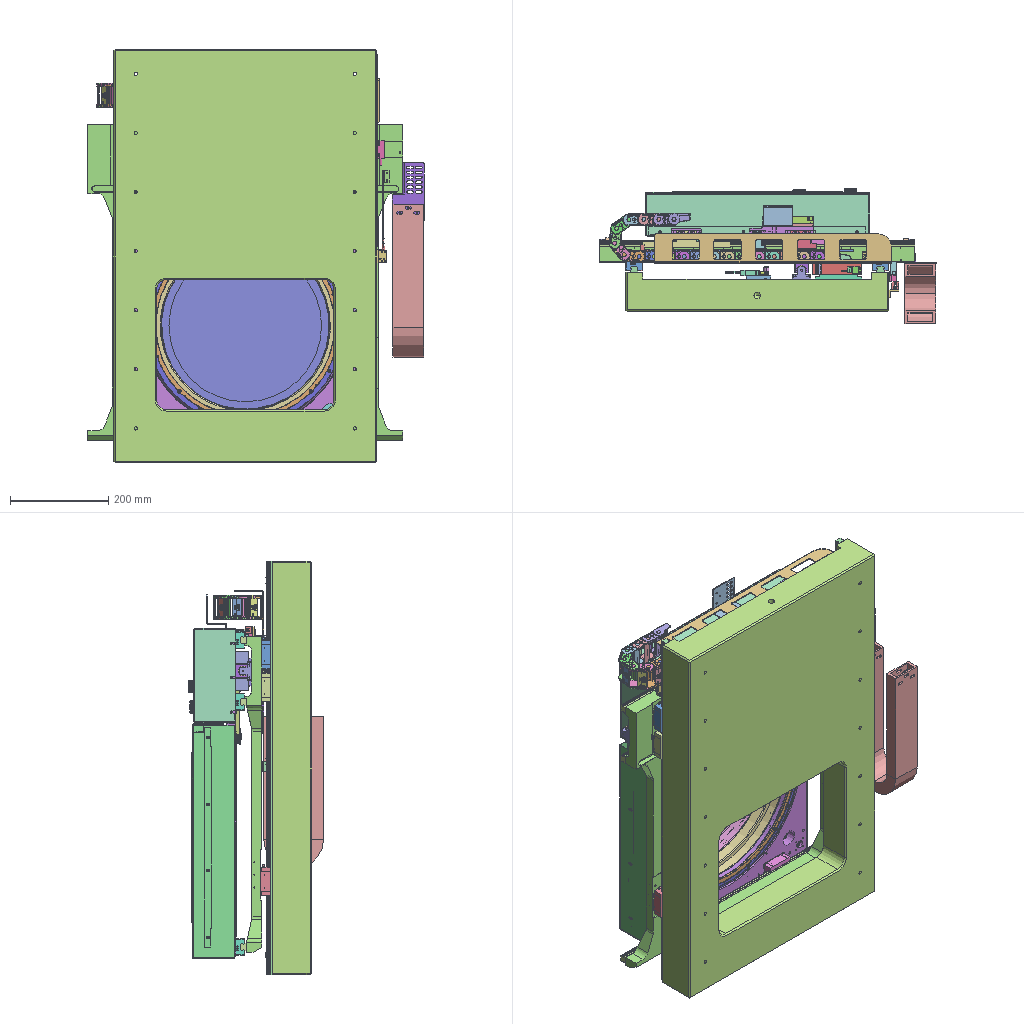Assembly | NX | 123 different items | 296 placed | box 684 x 274 x 840 mm
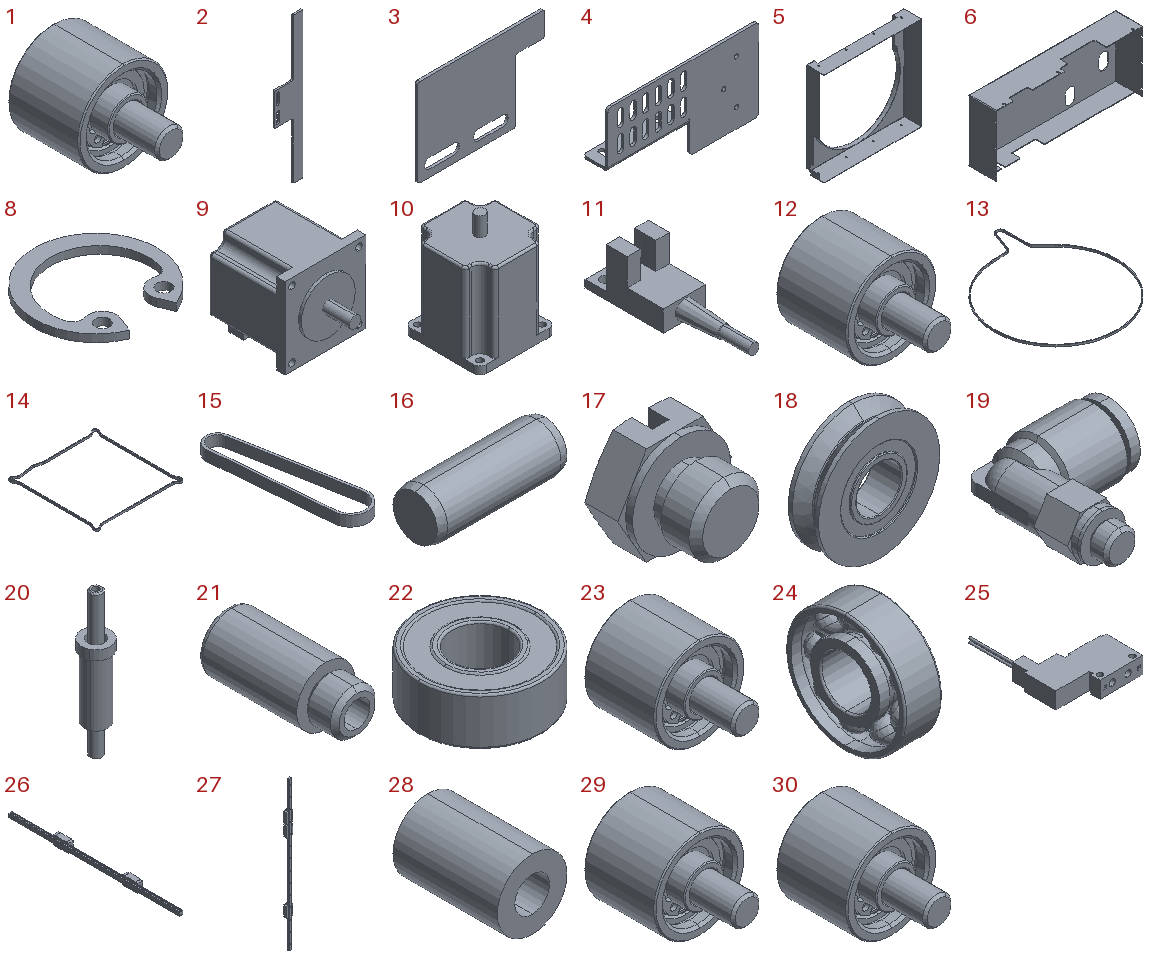Parts list (item | quantity | parent item | size | volume | features):
1 | x1 | in 56 | 19 x 27 x 19 mm | 4161 mm3 | features BREP 6
2 | x1 | in 56 | 35 x 2 x 180 mm | 5942 mm3 | features BREP 1
3 | x1 | in 56 | 52 x 1 x 36 mm | 1447 mm3 | features BREP 1
4 | x1 | in 50 | 120 x 20 x 65 mm | 13263 mm3 | features BREP 1
5 | x1 | in 34 | 477 x 86 x 455 mm | 309171 mm3 | features BREP 1
6 | x1 | in 34 | 456 x 85 x 191 mm | 341001 mm3 | features BREP 1
7 | x1 | in 48 | - | - | features BREP 42
8 | x11 | in 1, 12, 23, 29, 30, 31, 32, 33, 57, 59, 113 | 13 x 12.505 x 0.8 mm | 39.691 mm3 | features BREP 1
9 | x1 | in 62 | 57 x 90 x 65 mm | 164072 mm3 | features BREP 1
10 | x1 | in 35 | 60 x 60 x 105.1 mm | 217707 mm3 | features BREP 1
11 | x3 | in 49, 50 | 14 x 49 x 16 mm | 2990 mm3 | features BREP 1
12 | x1 | in 56 | 19 x 27 x 19 mm | 4161 mm3 | features BREP 6
13 | x1 | in 61 | 398.69 x 477.38 x 6 mm | 16623 mm3 | features BREP 1
14 | x1 | in 56 | 431.47 x 436.47 x 9 mm | 59188 mm3 | features BREP 1
15 | x1 | in 56 | 38.615 x 126.615 x 9 mm | 4997 mm3 | features BREP 1
16 | x6 | in 61 | 8 x 3 x 3 mm | 55.936 mm3 | features BREP 1
17 | x1 | in 64 | 8.083 x 6.5 x 7 mm | 172.44 mm3 | features BREP 1
18 | x10 | in 37, 38, 39, 40, 41, 42, 43, 44, 45, 46 | 16 x 4 x 16 mm | 572.042 mm3 | features BREP 1
19 | x1 | in 64 | 18.541 x 21.7 x 10.4 mm | 1291 mm3 | features BREP 1
20 | x4 | in 61 | 12 x 12 x 60 mm | 2642 mm3 | features BREP 2
21 | x1 | in 64 | 6.5 x 15 x 6.5 mm | 404.687 mm3 | features BREP 1
22 | x22 | in 1, 12, 23, 29, 30, 31, 32, 33, 57, 59, 60, 113 | 13 x 13 x 5 mm | 502.459 mm3 | features BREP 1
23 | x1 | in 56 | 19 x 27 x 19 mm | 4161 mm3 | features BREP 6
24 | x8 | in 52, 53, 54, 55 | 6 x 19 x 19 mm | 760.399 mm3 | features BREP 3
25 | x1 | in 64 | 49.5 x 69.5 x 11 mm | 13145 mm3 | features BREP 1
26 | x3 | in 50 | 24 x 640 x 34 mm | 168254 mm3 | features BREP 3
27 | x2 | in 49 | 34 x 24 x 840 mm | 231169 mm3 | features BREP 4
28 | x4 | in 102 | 8 x 12 x 8 mm | 452.389 mm3 | features BREP 1
29 | x1 | in 56 | 19 x 27 x 19 mm | 4161 mm3 | features BREP 6
30 | x1 | in 56 | 19 x 27 x 19 mm | 4161 mm3 | features BREP 6
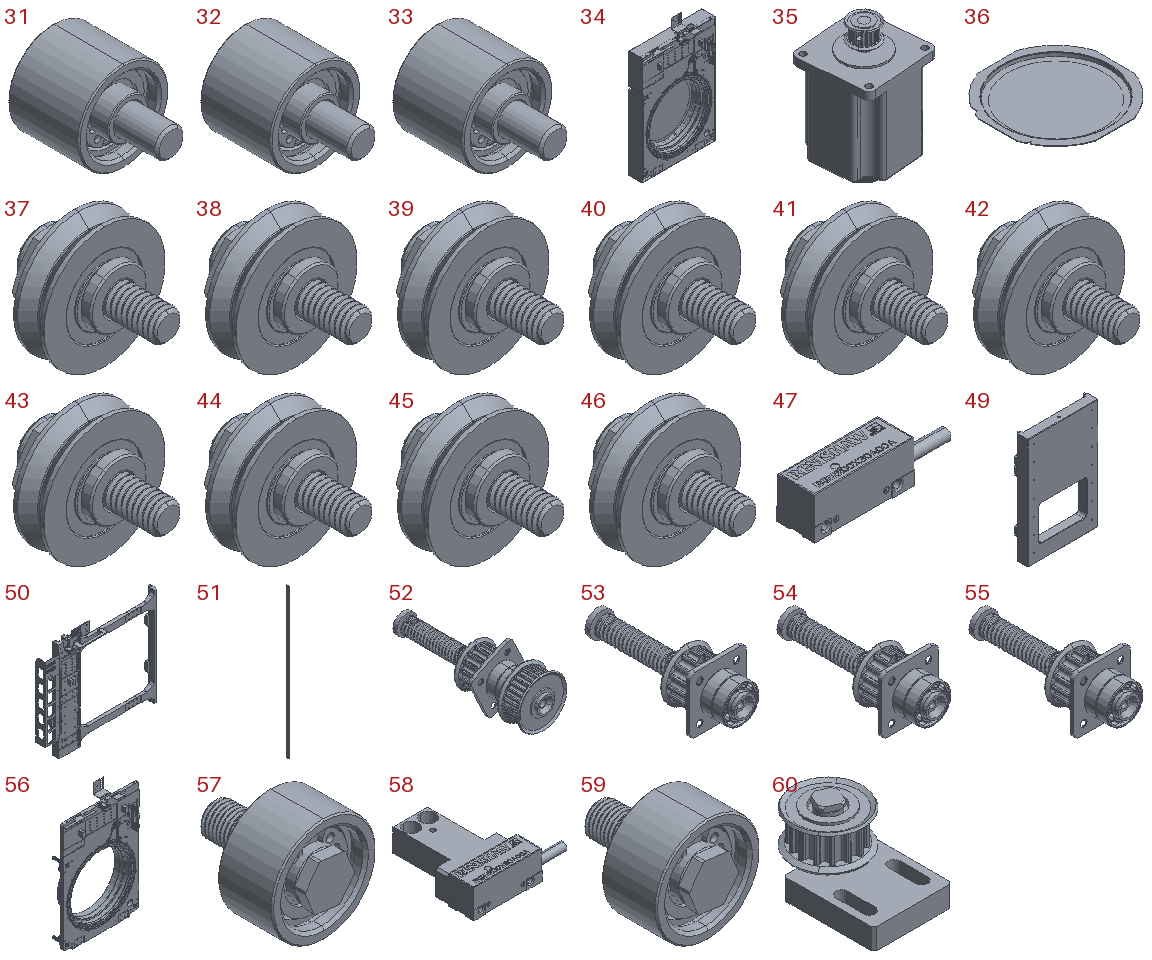31 | x1 | in 56 | 19 x 27 x 19 mm | 4161 mm3 | features BREP 6
32 | x1 | in 56 | 19 x 27 x 19 mm | 4161 mm3 | features BREP 6
33 | x1 | in 56 | 19 x 27 x 19 mm | 4161 mm3 | features BREP 6
34 | x1 | - | - | 6738834 mm3 | features BREP 68
35 | x1 | in 56 | 64.01 x 64.01 x 105.5 mm | 224733 mm3 | features BREP 3
36 | x1 | in 102 | 380 x 380 x 12.65 mm | 79362 mm3 | features BREP 2
37 | x1 | in 56 | 16 x 17 x 16 mm | 1088 mm3 | features BREP 4
38 | x1 | in 56 | 16 x 17 x 16 mm | 1088 mm3 | features BREP 4
39 | x1 | in 56 | 16 x 17 x 16 mm | 1088 mm3 | features BREP 4
40 | x1 | in 56 | 16 x 17 x 16 mm | 1088 mm3 | features BREP 4
41 | x1 | in 102 | 16 x 17 x 16 mm | 1088 mm3 | features BREP 4
42 | x1 | in 102 | 16 x 17 x 16 mm | 1088 mm3 | features BREP 4
43 | x1 | in 102 | 16 x 17 x 16 mm | 1088 mm3 | features BREP 4
44 | x1 | in 102 | 16 x 17 x 16 mm | 1088 mm3 | features BREP 4
45 | x1 | in 102 | 16 x 17 x 16 mm | 1088 mm3 | features BREP 4
46 | x1 | in 56 | 16 x 17 x 16 mm | 1088 mm3 | features BREP 4
47 | x2 | in 58, 69 | 50.65 x 13.5 x 14.8 mm | 6947 mm3 | features BREP 1
48 | x1 | - | - | - | features BREP 92
49 | x1 | in 48 | 555 x 105 x 840 mm | 24900873 mm3 | features BREP 22
50 | x1 | in 48 | - | 4255848 mm3 | features BREP 27
51 | x2 | in 49, 50 | 0.3 x 6 x 390 mm | 702 mm3 | features BREP 1
52 | x1 | in 56 | 37.314 x 92.5 x 37.314 mm | 18812 mm3 | features BREP 11
53 | x1 | in 56 | 29.5 x 77 x 29.5 mm | 11213 mm3 | features BREP 9
54 | x1 | in 56 | 29.5 x 77 x 29.5 mm | 11213 mm3 | features BREP 9
55 | x1 | in 56 | 29.5 x 77 x 29.5 mm | 11213 mm3 | features BREP 9
56 | x1 | in 34 | - | 4419914 mm3 | features BREP 53
57 | x1 | in 61 | 19 x 21 x 19 mm | 2699 mm3 | features BREP 6
58 | x1 | in 56 | 50.65 x 50.5 x 14.8 mm | 15333 mm3 | features BREP 2
59 | x1 | in 61 | 19 x 21 x 19 mm | 2699 mm3 | features BREP 6
60 | x1 | in 56 | 30 x 46 x 27.5 mm | 12594 mm3 | features BREP 6
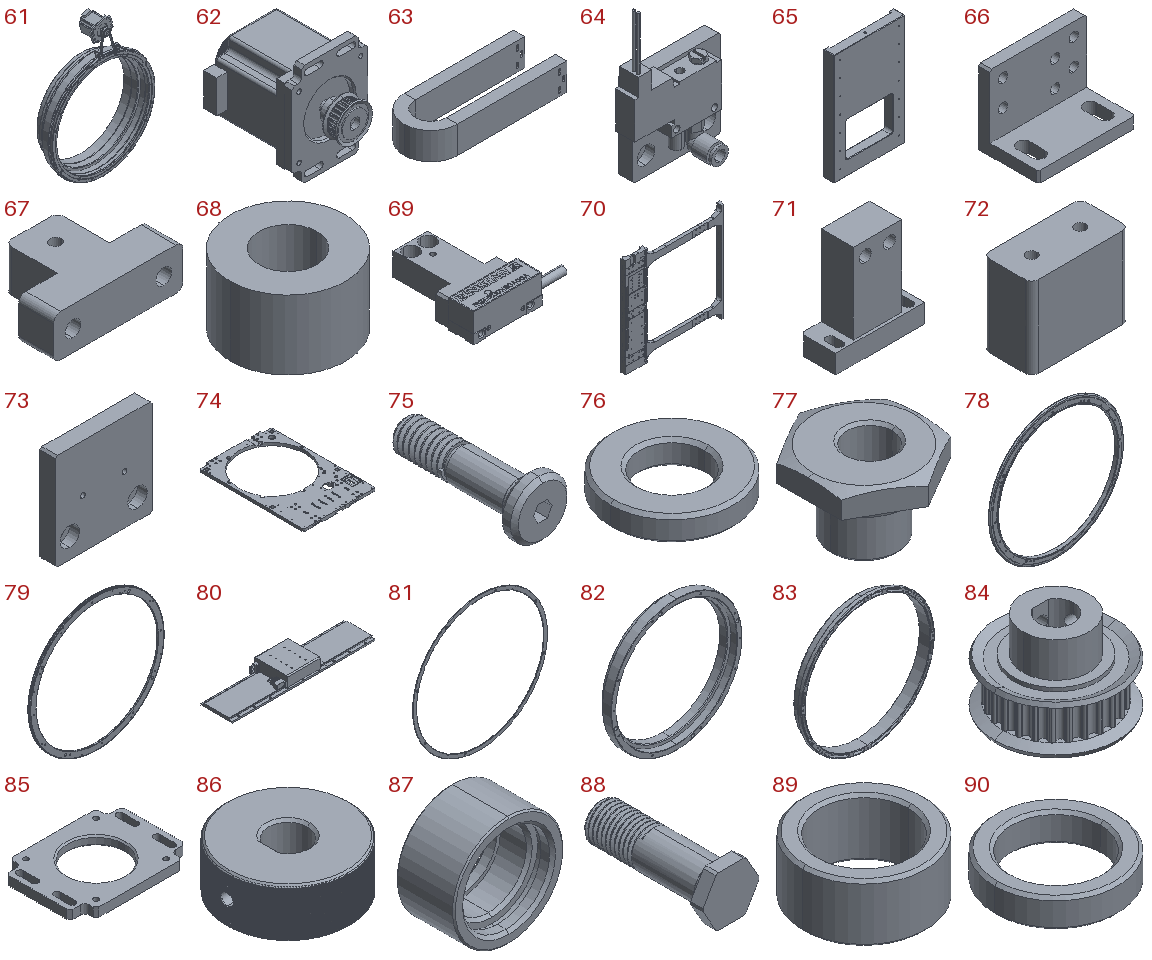61 | x1 | in 56 | - | 1411287 mm3 | features BREP 19
62 | x1 | in 61 | 65.5 x 93.95 x 78 mm | 190120 mm3 | features BREP 4
63 | x1 | in 48 | 310.75 x 121.5 x 62 mm | 440552 mm3 | features BREP 1
64 | x1 | in 48 | 59.75 x 28 x 92 mm | 34038 mm3 | features BREP 5
65 | x1 | in 49 | 535 x 79 x 840 mm | 23765456 mm3 | features BREP 1
66 | x3 | in 49, 50 | 26 x 16 x 20 mm | 2342 mm3 | features BREP 1
67 | x4 | in 49, 50 | 37 x 25 x 12 mm | 6187 mm3 | features BREP 1
68 | x4 | in 49, 50 | 20 x 20 x 12 mm | 3078 mm3 | features BREP 1
69 | x1 | in 50 | 50.65 x 50.5 x 14.8 mm | 15333 mm3 | features BREP 2
70 | x1 | in 50 | 642 x 34 x 640 mm | 2797211 mm3 | features BREP 1
71 | x2 | in 58, 69 | 33 x 13 x 37 mm | 8386 mm3 | features BREP 1
72 | x4 | in 50, 56 | 30 x 15 x 25 mm | 10986 mm3 | features BREP 1
73 | x1 | in 64 | 50 x 8 x 50 mm | 19025 mm3 | features BREP 1
74 | x1 | in 56 | 450 x 665 x 18 mm | 2551814 mm3 | features BREP 1
75 | x10 | in 37, 38, 39, 40, 41, 42, 43, 44, 45, 46 | 7 x 17 x 7 mm | 233.928 mm3 | features BREP 1
76 | x10 | in 37, 38, 39, 40, 41, 42, 43, 44, 45, 46 | 7.5 x 7.5 x 1.5 mm | 45.973 mm3 | features BREP 1
77 | x10 | in 37, 38, 39, 40, 41, 42, 43, 44, 45, 46 | 9.818 x 11.293 x 7 mm | 236.126 mm3 | features BREP 1
78 | x1 | in 61 | 408.8 x 11.6 x 408.8 mm | 208158 mm3 | features BREP 1
79 | x1 | in 61 | - | 89680 mm3 | features BREP 1
80 | x1 | in 49 | 431.8 x 100 x 40 mm | 648515 mm3 | features BREP 12
81 | x1 | in 61 | 402 x 2 x 402 mm | 25979 mm3 | features BREP 1
82 | x1 | in 61 | 393 x 42.5 x 393 mm | 727739 mm3 | features BREP 1
83 | x1 | in 61 | 363 x 30 x 363 mm | 137958 mm3 | features BREP 1
84 | x1 | in 62 | 28 x 28 x 19 mm | 5118 mm3 | features BREP 1
85 | x1 | in 62 | 78 x 58 x 6 mm | 16629 mm3 | features BREP 1
86 | x2 | in 35, 62 | 25 x 25 x 10 mm | 4302 mm3 | features BREP 1
87 | x2 | in 57, 59 | 19 x 10 x 19 mm | 1381 mm3 | features BREP 1
88 | x2 | in 57, 59 | 9 x 21 x 8.027 mm | 612.415 mm3 | features BREP 1
89 | x11 | in 1, 12, 23, 29, 30, 31, 32, 33, 57, 59, 113 | 8.5 x 8.5 x 4 mm | 108.247 mm3 | features BREP 1
90 | x2 | in 57, 59 | 8.5 x 8.5 x 2 mm | 53.206 mm3 | features BREP 1
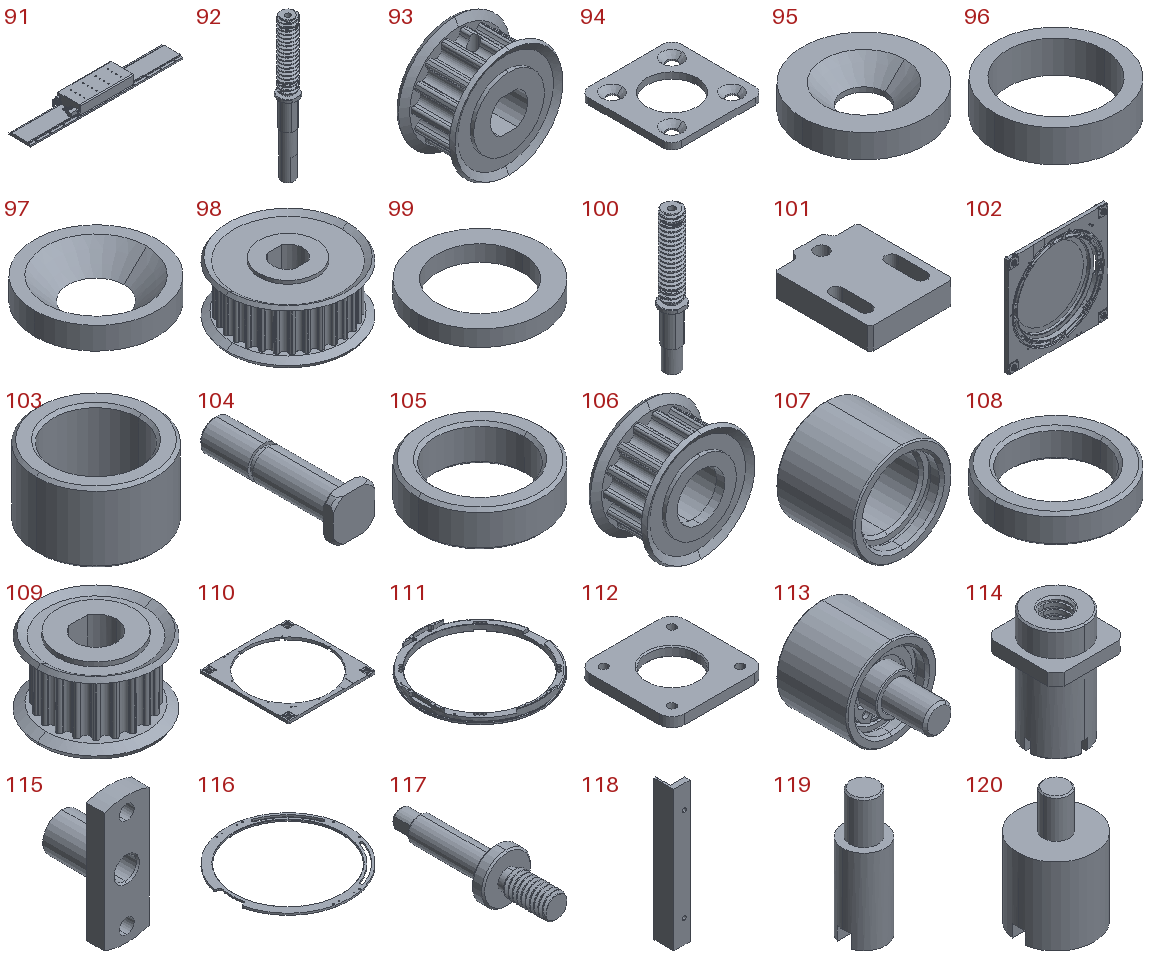91 | x1 | in 50 | 527.8 x 80 x 40 mm | 773171 mm3 | features BREP 12
92 | x1 | in 52 | 12 x 11 x 88 mm | 4646 mm3 | features BREP 1
93 | x4 | in 52, 53, 54, 55 | 27 x 14 x 27 mm | 4073 mm3 | features BREP 1
94 | x4 | in 52, 53, 54, 55 | 29.5 x 29.5 x 2 mm | 1183 mm3 | features BREP 1
95 | x4 | in 52, 53, 54, 55 | 13 x 13 x 2.5 mm | 255.418 mm3 | features BREP 1
96 | x4 | in 52, 53, 54, 55 | 11.5 x 11.5 x 3 mm | 120.755 mm3 | features BREP 1
97 | x4 | in 52, 53, 54, 55 | 11 x 11 x 2 mm | 111.003 mm3 | features BREP 1
98 | x1 | in 52 | 31.944 x 31.944 x 14 mm | 6821 mm3 | features BREP 1
99 | x1 | in 52 | 11.5 x 11.5 x 1.5 mm | 80.405 mm3 | features BREP 1
100 | x3 | in 53, 54, 55 | 12 x 11 x 72.3 mm | 3949 mm3 | features BREP 1
101 | x1 | in 60 | 30 x 37.5 x 8 mm | 7390 mm3 | features BREP 1
102 | x1 | in 34 | 450 x 46.9 x 455 mm | 1668771 mm3 | features BREP 17
103 | x1 | in 60 | 8.5 x 8.5 x 5 mm | 135.767 mm3 | features BREP 1
104 | x10 | in 1, 12, 23, 29, 30, 31, 32, 33, 60, 113 | 8 x 27 x 8 mm | 818.061 mm3 | features BREP 1
105 | x1 | in 60 | 8.5 x 8.5 x 2.5 mm | 66.966 mm3 | features BREP 1
106 | x1 | in 60 | 27 x 14 x 27 mm | 3178 mm3 | features BREP 1
107 | x9 | in 1, 12, 23, 29, 30, 31, 32, 33, 113 | 19 x 15 x 19 mm | 2137 mm3 | features BREP 1
108 | x9 | in 1, 12, 23, 29, 30, 31, 32, 33, 113 | 8.5 x 8.5 x 2 mm | 53.206 mm3 | features BREP 1
109 | x1 | in 35 | 23 x 23 x 14 mm | 2723 mm3 | features BREP 1
110 | x1 | in 102 | 450 x 455 x 15 mm | 943273 mm3 | features BREP 1
111 | x1 | in 102 | 415 x 415 x 33 mm | 391645 mm3 | features BREP 1
112 | x4 | in 102 | 39 x 39 x 4 mm | 4525 mm3 | features BREP 1
113 | x1 | in 56 | 19 x 27 x 19 mm | 4161 mm3 | features BREP 6
114 | x4 | in 102 | 23.7 x 23.7 x 37 mm | 6865 mm3 | features BREP 1
115 | x4 | in 102 | 10 x 14.5 x 28.5 mm | 1361 mm3 | features BREP 1
116 | x1 | in 102 | 403.128 x 409 x 6 mm | 160648 mm3 | features BREP 1
117 | x4 | in 102 | 8 x 25.5 x 8 mm | 353.749 mm3 | features BREP 1
118 | x2 | in 102 | 14 x 17 x 120 mm | 16235 mm3 | features BREP 1
119 | x1 | in 102 | 6 x 6 x 18 mm | 390.899 mm3 | features BREP 1
120 | x1 | in 102 | 11.8 x 11.8 x 18 mm | 1340 mm3 | features BREP 1
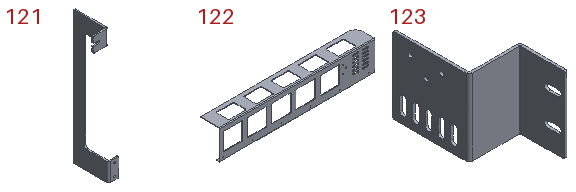121 | x1 | in 50 | 32 x 48 x 180 mm | 9470 mm3 | features BREP 1
122 | x1 | in 50 | 480 x 60 x 93 mm | 90767 mm3 | features BREP 1
123 | x1 | in 56 | 42 x 95 x 60 mm | 15058 mm3 | features BREP 1